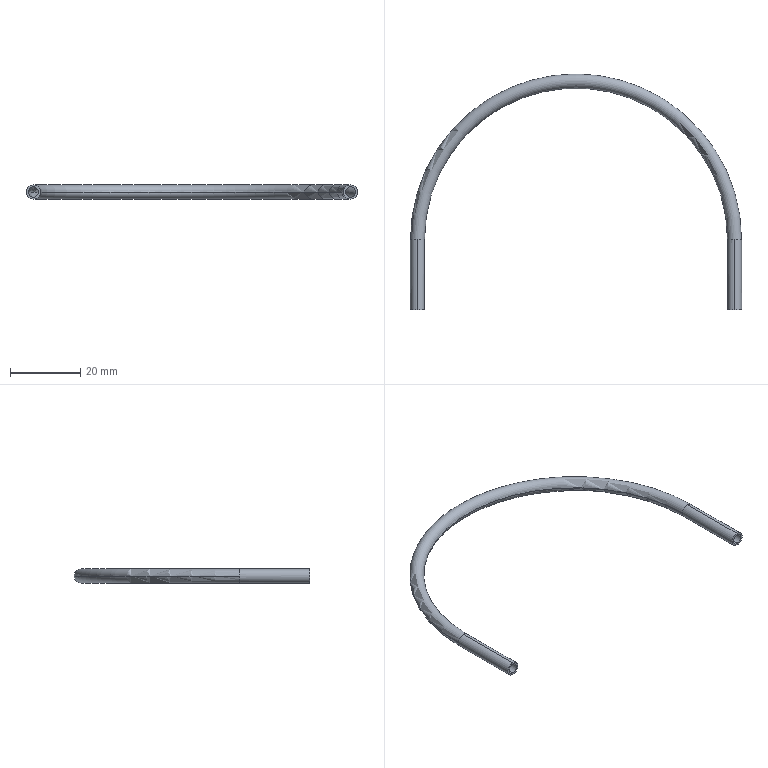Part | STEP file | 1 solid | 14 faces | box 94.3 x 67.15 x 4 mm | volume 999.734 mm3 | cylinder 8 | torus 4 | plane 2 | commonest cylinder face diameters 3 x4 4 x4
STEP:
#1=CARTESIAN_POINT('',(0.,0.,0.));
#2=DIRECTION('',(0.,0.,1.));
#3=DIRECTION('',(1.,0.,0.));
#4=AXIS2_PLACEMENT_3D('',#1,#2,#3);
#5=CARTESIAN_POINT('',(45.15,0.,-2.));
#6=VERTEX_POINT('',#5);
#7=CARTESIAN_POINT('',(45.15,20.,-2.));
#8=VERTEX_POINT('',#7);
#9=CARTESIAN_POINT('',(45.15,0.,-2.));
#10=DIRECTION('',(0.,1.,0.));
#11=VECTOR('',#10,1.);
#12=LINE('',#9,#11);
#13=CARTESIAN_POINT('',(45.15,0.,0.));
#14=DIRECTION('',(0.,1.,0.));
#15=DIRECTION('',(0.,0.,1.));
#16=AXIS2_PLACEMENT_3D('',#13,#14,#15);
#17=CYLINDRICAL_SURFACE('',#16,2.);
#18=CARTESIAN_POINT('',(3.142,0.));
#19=DIRECTION('',(0.,1.));
#20=VECTOR('',#19,1.);
#21=LINE('',#18,#20);
#22=(GEOMETRIC_REPRESENTATION_CONTEXT(2)PARAMETRIC_REPRESENTATION_CONTEXT()REPRESENTATION_CONTEXT('',''));
#23=DEFINITIONAL_REPRESENTATION('',(#21),#22);
#24=PCURVE('',#17,#23);
#25=CARTESIAN_POINT('',(45.15,0.,0.));
#26=DIRECTION('',(0.,1.,0.));
#27=DIRECTION('',(0.,0.,1.));
#28=AXIS2_PLACEMENT_3D('',#25,#26,#27);
#29=CYLINDRICAL_SURFACE('',#28,2.);
#30=CARTESIAN_POINT('',(3.142,0.));
#31=DIRECTION('',(0.,1.));
#32=VECTOR('',#31,1.);
#33=LINE('',#30,#32);
#34=(GEOMETRIC_REPRESENTATION_CONTEXT(2)PARAMETRIC_REPRESENTATION_CONTEXT()REPRESENTATION_CONTEXT('',''));
#35=DEFINITIONAL_REPRESENTATION('',(#33),#34);
#36=PCURVE('',#29,#35);
#37=SURFACE_CURVE('',#12,(#24,#36),.PCURVE_S1.);
#38=EDGE_CURVE('',#6,#8,#37,.T.);
#39=ORIENTED_EDGE('',*,*,#38,.F.);
#40=CARTESIAN_POINT('',(45.15,0.,2.));
#41=VERTEX_POINT('',#40);
#42=CARTESIAN_POINT('',(45.15,0.,0.));
#43=DIRECTION('',(0.,-1.,0.));
#44=DIRECTION('',(0.,0.,1.));
#45=AXIS2_PLACEMENT_3D('',#42,#43,#44);
#46=CIRCLE('',#45,2.);
#47=CARTESIAN_POINT('',(6.283,0.));
#48=DIRECTION('',(-1.,0.));
#49=VECTOR('',#48,1.);
#50=LINE('',#47,#49);
#51=(GEOMETRIC_REPRESENTATION_CONTEXT(2)PARAMETRIC_REPRESENTATION_CONTEXT()REPRESENTATION_CONTEXT('',''));
#52=DEFINITIONAL_REPRESENTATION('',(#50),#51);
#53=PCURVE('',#17,#52);
#54=CARTESIAN_POINT('',(45.15,0.,0.));
#55=DIRECTION('',(0.,-1.,0.));
#56=DIRECTION('',(0.,0.,1.));
#57=AXIS2_PLACEMENT_3D('',#54,#55,#56);
#58=PLANE('',#57);
#59=CARTESIAN_POINT('',(0.,0.));
#60=DIRECTION('',(1.,0.));
#61=AXIS2_PLACEMENT_2D('',#59,#60);
#62=CIRCLE('',#61,2.);
#63=(GEOMETRIC_REPRESENTATION_CONTEXT(2)PARAMETRIC_REPRESENTATION_CONTEXT()REPRESENTATION_CONTEXT('',''));
#64=DEFINITIONAL_REPRESENTATION('',(#62),#63);
#65=PCURVE('',#58,#64);
#66=SURFACE_CURVE('',#46,(#53,#65),.PCURVE_S1.);
#67=EDGE_CURVE('',#41,#6,#66,.T.);
#68=ORIENTED_EDGE('',*,*,#67,.F.);
#69=CARTESIAN_POINT('',(45.15,20.,2.));
#70=VERTEX_POINT('',#69);
#71=CARTESIAN_POINT('',(45.15,0.,2.));
#72=DIRECTION('',(0.,1.,0.));
#73=VECTOR('',#72,1.);
#74=LINE('',#71,#73);
#75=CARTESIAN_POINT('',(6.283,0.));
#76=DIRECTION('',(0.,1.));
#77=VECTOR('',#76,1.);
#78=LINE('',#75,#77);
#79=(GEOMETRIC_REPRESENTATION_CONTEXT(2)PARAMETRIC_REPRESENTATION_CONTEXT()REPRESENTATION_CONTEXT('',''));
#80=DEFINITIONAL_REPRESENTATION('',(#78),#79);
#81=PCURVE('',#17,#80);
#82=CARTESIAN_POINT('',(0.,0.));
#83=DIRECTION('',(0.,1.));
#84=VECTOR('',#83,1.);
#85=LINE('',#82,#84);
#86=(GEOMETRIC_REPRESENTATION_CONTEXT(2)PARAMETRIC_REPRESENTATION_CONTEXT()REPRESENTATION_CONTEXT('',''));
#87=DEFINITIONAL_REPRESENTATION('',(#85),#86);
#88=PCURVE('',#29,#87);
#89=SURFACE_CURVE('',#74,(#81,#88),.PCURVE_S1.);
#90=EDGE_CURVE('',#41,#70,#89,.T.);
#91=ORIENTED_EDGE('',*,*,#90,.T.);
#92=CARTESIAN_POINT('',(43.15,20.,0.));
#93=VERTEX_POINT('',#92);
#94=CARTESIAN_POINT('',(45.15,20.,0.));
#95=DIRECTION('',(0.,-1.,0.));
#96=DIRECTION('',(0.,0.,1.));
#97=AXIS2_PLACEMENT_3D('',#94,#95,#96);
#98=CIRCLE('',#97,2.);
#99=CARTESIAN_POINT('',(6.283,20.));
#100=DIRECTION('',(-1.,0.));
#101=VECTOR('',#100,1.);
#102=LINE('',#99,#101);
#103=(GEOMETRIC_REPRESENTATION_CONTEXT(2)PARAMETRIC_REPRESENTATION_CONTEXT()REPRESENTATION_CONTEXT('',''));
#104=DEFINITIONAL_REPRESENTATION('',(#102),#103);
#105=PCURVE('',#17,#104);
#106=CARTESIAN_POINT('',(0.,20.,0.));
#107=DIRECTION('',(0.,0.,1.));
#108=DIRECTION('',(1.,0.,0.));
#109=AXIS2_PLACEMENT_3D('',#106,#107,#108);
#110=TOROIDAL_SURFACE('',#109,45.15,2.);
#111=CARTESIAN_POINT('',(0.,1.571));
#112=DIRECTION('',(0.,1.));
#113=VECTOR('',#112,1.);
#114=LINE('',#111,#113);
#115=(GEOMETRIC_REPRESENTATION_CONTEXT(2)PARAMETRIC_REPRESENTATION_CONTEXT()REPRESENTATION_CONTEXT('',''));
#116=DEFINITIONAL_REPRESENTATION('',(#114),#115);
#117=PCURVE('',#110,#116);
#118=SURFACE_CURVE('',#98,(#105,#117),.PCURVE_S1.);
#119=EDGE_CURVE('',#70,#93,#118,.T.);
#120=ORIENTED_EDGE('',*,*,#119,.T.);
#121=CARTESIAN_POINT('',(45.15,20.,0.));
#122=DIRECTION('',(0.,-1.,0.));
#123=DIRECTION('',(0.,0.,1.));
#124=AXIS2_PLACEMENT_3D('',#121,#122,#123);
#125=CIRCLE('',#124,2.);
#126=CARTESIAN_POINT('',(6.283,20.));
#127=DIRECTION('',(-1.,0.));
#128=VECTOR('',#127,1.);
#129=LINE('',#126,#128);
#130=(GEOMETRIC_REPRESENTATION_CONTEXT(2)PARAMETRIC_REPRESENTATION_CONTEXT()REPRESENTATION_CONTEXT('',''));
#131=DEFINITIONAL_REPRESENTATION('',(#129),#130);
#132=PCURVE('',#17,#131);
#133=CARTESIAN_POINT('',(0.,20.,0.));
#134=DIRECTION('',(0.,0.,1.));
#135=DIRECTION('',(1.,0.,0.));
#136=AXIS2_PLACEMENT_3D('',#133,#134,#135);
#137=TOROIDAL_SURFACE('',#136,45.15,2.);
#138=CARTESIAN_POINT('',(0.,1.571));
#139=DIRECTION('',(0.,1.));
#140=VECTOR('',#139,1.);
#141=LINE('',#138,#140);
#142=(GEOMETRIC_REPRESENTATION_CONTEXT(2)PARAMETRIC_REPRESENTATION_CONTEXT()REPRESENTATION_CONTEXT('',''));
#143=DEFINITIONAL_REPRESENTATION('',(#141),#142);
#144=PCURVE('',#137,#143);
#145=SURFACE_CURVE('',#125,(#132,#144),.PCURVE_S1.);
#146=EDGE_CURVE('',#93,#8,#145,.T.);
#147=ORIENTED_EDGE('',*,*,#146,.T.);
#148=EDGE_LOOP('',(#39,#68,#91,#120,#147));
#149=FACE_BOUND('',#148,.T.);
#150=ADVANCED_FACE('',(#149),#17,.T.);
#151=CARTESIAN_POINT('',(47.15,20.,0.));
#152=VERTEX_POINT('',#151);
#153=CARTESIAN_POINT('',(-47.15,20.,0.));
#154=VERTEX_POINT('',#153);
#155=CARTESIAN_POINT('',(0.,20.,0.));
#156=DIRECTION('',(0.,0.,1.));
#157=DIRECTION('',(1.,0.,0.));
#158=AXIS2_PLACEMENT_3D('',#155,#156,#157);
#159=CIRCLE('',#158,47.15);
#160=CARTESIAN_POINT('',(0.,6.283));
#161=DIRECTION('',(1.,0.));
#162=VECTOR('',#161,1.);
#163=LINE('',#160,#162);
#164=(GEOMETRIC_REPRESENTATION_CONTEXT(2)PARAMETRIC_REPRESENTATION_CONTEXT()REPRESENTATION_CONTEXT('',''));
#165=DEFINITIONAL_REPRESENTATION('',(#163),#164);
#166=PCURVE('',#137,#165);
#167=CARTESIAN_POINT('',(0.,0.));
#168=DIRECTION('',(1.,0.));
#169=VECTOR('',#168,1.);
#170=LINE('',#167,#169);
#171=(GEOMETRIC_REPRESENTATION_CONTEXT(2)PARAMETRIC_REPRESENTATION_CONTEXT()REPRESENTATION_CONTEXT('',''));
#172=DEFINITIONAL_REPRESENTATION('',(#170),#171);
#173=PCURVE('',#110,#172);
#174=SURFACE_CURVE('',#159,(#166,#173),.PCURVE_S1.);
#175=EDGE_CURVE('',#152,#154,#174,.T.);
#176=ORIENTED_EDGE('',*,*,#175,.F.);
#177=CARTESIAN_POINT('',(45.15,20.,0.));
#178=DIRECTION('',(0.,-1.,0.));
#179=DIRECTION('',(0.,0.,1.));
#180=AXIS2_PLACEMENT_3D('',#177,#178,#179);
#181=CIRCLE('',#180,2.);
#182=CARTESIAN_POINT('',(0.,1.571));
#183=DIRECTION('',(0.,1.));
#184=VECTOR('',#183,1.);
#185=LINE('',#182,#184);
#186=(GEOMETRIC_REPRESENTATION_CONTEXT(2)PARAMETRIC_REPRESENTATION_CONTEXT()REPRESENTATION_CONTEXT('',''));
#187=DEFINITIONAL_REPRESENTATION('',(#185),#186);
#188=PCURVE('',#137,#187);
#189=CARTESIAN_POINT('',(6.283,20.));
#190=DIRECTION('',(-1.,0.));
#191=VECTOR('',#190,1.);
#192=LINE('',#189,#191);
#193=(GEOMETRIC_REPRESENTATION_CONTEXT(2)PARAMETRIC_REPRESENTATION_CONTEXT()REPRESENTATION_CONTEXT('',''));
#194=DEFINITIONAL_REPRESENTATION('',(#192),#193);
#195=PCURVE('',#29,#194);
#196=SURFACE_CURVE('',#181,(#188,#195),.PCURVE_S1.);
#197=EDGE_CURVE('',#8,#152,#196,.T.);
#198=ORIENTED_EDGE('',*,*,#197,.F.);
#199=ORIENTED_EDGE('',*,*,#146,.F.);
#200=CARTESIAN_POINT('',(-43.15,20.,0.));
#201=VERTEX_POINT('',#200);
#202=CARTESIAN_POINT('',(0.,20.,0.));
#203=DIRECTION('',(0.,0.,1.));
#204=DIRECTION('',(1.,0.,0.));
#205=AXIS2_PLACEMENT_3D('',#202,#203,#204);
#206=CIRCLE('',#205,43.15);
#207=CARTESIAN_POINT('',(0.,3.142));
#208=DIRECTION('',(1.,0.));
#209=VECTOR('',#208,1.);
#210=LINE('',#207,#209);
#211=(GEOMETRIC_REPRESENTATION_CONTEXT(2)PARAMETRIC_REPRESENTATION_CONTEXT()REPRESENTATION_CONTEXT('',''));
#212=DEFINITIONAL_REPRESENTATION('',(#210),#211);
#213=PCURVE('',#137,#212);
#214=CARTESIAN_POINT('',(0.,3.142));
#215=DIRECTION('',(1.,0.));
#216=VECTOR('',#215,1.);
#217=LINE('',#214,#216);
#218=(GEOMETRIC_REPRESENTATION_CONTEXT(2)PARAMETRIC_REPRESENTATION_CONTEXT()REPRESENTATION_CONTEXT('',''));
#219=DEFINITIONAL_REPRESENTATION('',(#217),#218);
#220=PCURVE('',#110,#219);
#221=SURFACE_CURVE('',#206,(#213,#220),.PCURVE_S1.);
#222=EDGE_CURVE('',#93,#201,#221,.T.);
#223=ORIENTED_EDGE('',*,*,#222,.T.);
#224=CARTESIAN_POINT('',(-45.15,20.,-2.));
#225=VERTEX_POINT('',#224);
#226=CARTESIAN_POINT('',(-45.15,20.,0.));
#227=DIRECTION('',(0.,1.,0.));
#228=DIRECTION('',(0.,0.,1.));
#229=AXIS2_PLACEMENT_3D('',#226,#227,#228);
#230=CIRCLE('',#229,2.);
#231=CARTESIAN_POINT('',(3.142,1.571));
#232=DIRECTION('',(0.,1.));
#233=VECTOR('',#232,1.);
#234=LINE('',#231,#233);
#235=(GEOMETRIC_REPRESENTATION_CONTEXT(2)PARAMETRIC_REPRESENTATION_CONTEXT()REPRESENTATION_CONTEXT('',''));
#236=DEFINITIONAL_REPRESENTATION('',(#234),#235);
#237=PCURVE('',#137,#236);
#238=CARTESIAN_POINT('',(-45.15,20.,0.));
#239=DIRECTION('',(0.,-1.,0.));
#240=DIRECTION('',(0.,0.,-1.));
#241=AXIS2_PLACEMENT_3D('',#238,#239,#240);
#242=CYLINDRICAL_SURFACE('',#241,2.);
#243=CARTESIAN_POINT('',(3.142,0.));
#244=DIRECTION('',(-1.,0.));
#245=VECTOR('',#244,1.);
#246=LINE('',#243,#245);
#247=(GEOMETRIC_REPRESENTATION_CONTEXT(2)PARAMETRIC_REPRESENTATION_CONTEXT()REPRESENTATION_CONTEXT('',''));
#248=DEFINITIONAL_REPRESENTATION('',(#246),#247);
#249=PCURVE('',#242,#248);
#250=SURFACE_CURVE('',#230,(#237,#249),.PCURVE_S1.);
#251=EDGE_CURVE('',#201,#225,#250,.T.);
#252=ORIENTED_EDGE('',*,*,#251,.T.);
#253=CARTESIAN_POINT('',(-45.15,20.,0.));
#254=DIRECTION('',(0.,1.,0.));
#255=DIRECTION('',(0.,0.,1.));
#256=AXIS2_PLACEMENT_3D('',#253,#254,#255);
#257=CIRCLE('',#256,2.);
#258=CARTESIAN_POINT('',(3.142,1.571));
#259=DIRECTION('',(0.,1.));
#260=VECTOR('',#259,1.);
#261=LINE('',#258,#260);
#262=(GEOMETRIC_REPRESENTATION_CONTEXT(2)PARAMETRIC_REPRESENTATION_CONTEXT()REPRESENTATION_CONTEXT('',''));
#263=DEFINITIONAL_REPRESENTATION('',(#261),#262);
#264=PCURVE('',#137,#263);
#265=CARTESIAN_POINT('',(-45.15,20.,0.));
#266=DIRECTION('',(0.,-1.,0.));
#267=DIRECTION('',(0.,0.,-1.));
#268=AXIS2_PLACEMENT_3D('',#265,#266,#267);
#269=CYLINDRICAL_SURFACE('',#268,2.);
#270=CARTESIAN_POINT('',(9.425,0.));
#271=DIRECTION('',(-1.,0.));
#272=VECTOR('',#271,1.);
#273=LINE('',#270,#272);
#274=(GEOMETRIC_REPRESENTATION_CONTEXT(2)PARAMETRIC_REPRESENTATION_CONTEXT()REPRESENTATION_CONTEXT('',''));
#275=DEFINITIONAL_REPRESENTATION('',(#273),#274);
#276=PCURVE('',#269,#275);
#277=SURFACE_CURVE('',#257,(#264,#276),.PCURVE_S1.);
#278=EDGE_CURVE('',#225,#154,#277,.T.);
#279=ORIENTED_EDGE('',*,*,#278,.T.);
#280=EDGE_LOOP('',(#176,#198,#199,#223,#252,#279));
#281=FACE_BOUND('',#280,.T.);
#282=ADVANCED_FACE('',(#281),#137,.T.);
#283=CARTESIAN_POINT('',(-45.15,20.,2.));
#284=VERTEX_POINT('',#283);
#285=CARTESIAN_POINT('',(-45.15,0.,2.));
#286=VERTEX_POINT('',#285);
#287=CARTESIAN_POINT('',(-45.15,20.,2.));
#288=DIRECTION('',(0.,-1.,0.));
#289=VECTOR('',#288,1.);
#290=LINE('',#287,#289);
#291=CARTESIAN_POINT('',(3.142,0.));
#292=DIRECTION('',(0.,1.));
#293=VECTOR('',#292,1.);
#294=LINE('',#291,#293);
#295=(GEOMETRIC_REPRESENTATION_CONTEXT(2)PARAMETRIC_REPRESENTATION_CONTEXT()REPRESENTATION_CONTEXT('',''));
#296=DEFINITIONAL_REPRESENTATION('',(#294),#295);
#297=PCURVE('',#269,#296);
#298=CARTESIAN_POINT('',(3.142,0.));
#299=DIRECTION('',(0.,1.));
#300=VECTOR('',#299,1.);
#301=LINE('',#298,#300);
#302=(GEOMETRIC_REPRESENTATION_CONTEXT(2)PARAMETRIC_REPRESENTATION_CONTEXT()REPRESENTATION_CONTEXT('',''));
#303=DEFINITIONAL_REPRESENTATION('',(#301),#302);
#304=PCURVE('',#242,#303);
#305=SURFACE_CURVE('',#290,(#297,#304),.PCURVE_S1.);
#306=EDGE_CURVE('',#284,#286,#305,.T.);
#307=ORIENTED_EDGE('',*,*,#306,.F.);
#308=CARTESIAN_POINT('',(-45.15,20.,0.));
#309=DIRECTION('',(0.,1.,0.));
#310=DIRECTION('',(0.,0.,1.));
#311=AXIS2_PLACEMENT_3D('',#308,#309,#310);
#312=CIRCLE('',#311,2.);
#313=CARTESIAN_POINT('',(9.425,0.));
#314=DIRECTION('',(-1.,0.));
#315=VECTOR('',#314,1.);
#316=LINE('',#313,#315);
#317=(GEOMETRIC_REPRESENTATION_CONTEXT(2)PARAMETRIC_REPRESENTATION_CONTEXT()REPRESENTATION_CONTEXT('',''));
#318=DEFINITIONAL_REPRESENTATION('',(#316),#317);
#319=PCURVE('',#269,#318);
#320=CARTESIAN_POINT('',(3.142,-4.712));
#321=DIRECTION('',(0.,1.));
#322=VECTOR('',#321,1.);
#323=LINE('',#320,#322);
#324=(GEOMETRIC_REPRESENTATION_CONTEXT(2)PARAMETRIC_REPRESENTATION_CONTEXT()REPRESENTATION_CONTEXT('',''));
#325=DEFINITIONAL_REPRESENTATION('',(#323),#324);
#326=PCURVE('',#110,#325);
#327=SURFACE_CURVE('',#312,(#319,#326),.PCURVE_S1.);
#328=EDGE_CURVE('',#154,#284,#327,.T.);
#329=ORIENTED_EDGE('',*,*,#328,.F.);
#330=ORIENTED_EDGE('',*,*,#278,.F.);
#331=CARTESIAN_POINT('',(-45.15,0.,-2.));
#332=VERTEX_POINT('',#331);
#333=CARTESIAN_POINT('',(-45.15,20.,-2.));
#334=DIRECTION('',(0.,-1.,0.));
#335=VECTOR('',#334,1.);
#336=LINE('',#333,#335);
#337=CARTESIAN_POINT('',(6.283,0.));
#338=DIRECTION('',(0.,1.));
#339=VECTOR('',#338,1.);
#340=LINE('',#337,#339);
#341=(GEOMETRIC_REPRESENTATION_CONTEXT(2)PARAMETRIC_REPRESENTATION_CONTEXT()REPRESENTATION_CONTEXT('',''));
#342=DEFINITIONAL_REPRESENTATION('',(#340),#341);
#343=PCURVE('',#269,#342);
#344=CARTESIAN_POINT('',(0.,0.));
#345=DIRECTION('',(0.,1.));
#346=VECTOR('',#345,1.);
#347=LINE('',#344,#346);
#348=(GEOMETRIC_REPRESENTATION_CONTEXT(2)PARAMETRIC_REPRESENTATION_CONTEXT()REPRESENTATION_CONTEXT('',''));
#349=DEFINITIONAL_REPRESENTATION('',(#347),#348);
#350=PCURVE('',#242,#349);
#351=SURFACE_CURVE('',#336,(#343,#350),.PCURVE_S1.);
#352=EDGE_CURVE('',#225,#332,#351,.T.);
#353=ORIENTED_EDGE('',*,*,#352,.T.);
#354=CARTESIAN_POINT('',(-45.15,0.,0.));
#355=DIRECTION('',(0.,1.,0.));
#356=DIRECTION('',(0.,0.,1.));
#357=AXIS2_PLACEMENT_3D('',#354,#355,#356);
#358=CIRCLE('',#357,2.);
#359=CARTESIAN_POINT('',(9.425,20.));
#360=DIRECTION('',(-1.,0.));
#361=VECTOR('',#360,1.);
#362=LINE('',#359,#361);
#363=(GEOMETRIC_REPRESENTATION_CONTEXT(2)PARAMETRIC_REPRESENTATION_CONTEXT()REPRESENTATION_CONTEXT('',''));
#364=DEFINITIONAL_REPRESENTATION('',(#362),#363);
#365=PCURVE('',#269,#364);
#366=CARTESIAN_POINT('',(-45.15,0.,0.));
#367=DIRECTION('',(0.,1.,0.));
#368=DIRECTION('',(0.,0.,1.));
#369=AXIS2_PLACEMENT_3D('',#366,#367,#368);
#370=PLANE('',#369);
#371=CARTESIAN_POINT('',(0.,0.));
#372=DIRECTION('',(1.,0.));
#373=AXIS2_PLACEMENT_2D('',#371,#372);
#374=CIRCLE('',#373,2.);
#375=(GEOMETRIC_REPRESENTATION_CONTEXT(2)PARAMETRIC_REPRESENTATION_CONTEXT()REPRESENTATION_CONTEXT('',''));
#376=DEFINITIONAL_REPRESENTATION('',(#374),#375);
#377=PCURVE('',#370,#376);
#378=SURFACE_CURVE('',#358,(#365,#377),.PCURVE_S1.);
#379=EDGE_CURVE('',#332,#286,#378,.T.);
#380=ORIENTED_EDGE('',*,*,#379,.T.);
#381=EDGE_LOOP('',(#307,#329,#330,#353,#380));
#382=FACE_BOUND('',#381,.T.);
#383=ADVANCED_FACE('',(#382),#269,.T.);
#384=ORIENTED_EDGE('',*,*,#67,.T.);
#385=CARTESIAN_POINT('',(45.15,0.,0.));
#386=DIRECTION('',(0.,-1.,0.));
#387=DIRECTION('',(0.,0.,1.));
#388=AXIS2_PLACEMENT_3D('',#385,#386,#387);
#389=CIRCLE('',#388,2.);
#390=CARTESIAN_POINT('',(0.,0.));
#391=DIRECTION('',(1.,0.));
#392=AXIS2_PLACEMENT_2D('',#390,#391);
#393=CIRCLE('',#392,2.);
#394=(GEOMETRIC_REPRESENTATION_CONTEXT(2)PARAMETRIC_REPRESENTATION_CONTEXT()REPRESENTATION_CONTEXT('',''));
#395=DEFINITIONAL_REPRESENTATION('',(#393),#394);
#396=PCURVE('',#58,#395);
#397=CARTESIAN_POINT('',(6.283,0.));
#398=DIRECTION('',(-1.,0.));
#399=VECTOR('',#398,1.);
#400=LINE('',#397,#399);
#401=(GEOMETRIC_REPRESENTATION_CONTEXT(2)PARAMETRIC_REPRESENTATION_CONTEXT()REPRESENTATION_CONTEXT('',''));
#402=DEFINITIONAL_REPRESENTATION('',(#400),#401);
#403=PCURVE('',#29,#402);
#404=SURFACE_CURVE('',#389,(#396,#403),.PCURVE_S1.);
#405=EDGE_CURVE('',#6,#41,#404,.T.);
#406=ORIENTED_EDGE('',*,*,#405,.T.);
#407=EDGE_LOOP('',(#384,#406));
#408=FACE_BOUND('',#407,.T.);
#409=CARTESIAN_POINT('',(45.15,0.,1.5));
#410=VERTEX_POINT('',#409);
#411=CARTESIAN_POINT('',(45.15,0.,-1.5));
#412=VERTEX_POINT('',#411);
#413=CARTESIAN_POINT('',(45.15,0.,0.));
#414=DIRECTION('',(0.,1.,0.));
#415=DIRECTION('',(0.,0.,1.));
#416=AXIS2_PLACEMENT_3D('',#413,#414,#415);
#417=CIRCLE('',#416,1.5);
#418=CARTESIAN_POINT('',(1.5,0.));
#419=CARTESIAN_POINT('',(1.5,-2.598));
#420=CARTESIAN_POINT('',(-0.75,-1.299));
#421=CARTESIAN_POINT('',(-3.,0.));
#422=CARTESIAN_POINT('',(-0.75,1.299));
#423=CARTESIAN_POINT('',(1.5,2.598));
#424=CARTESIAN_POINT('',(1.5,0.));
#425=(BOUNDED_CURVE()B_SPLINE_CURVE(2,(#418,#419,#420,#421,#422,#423,#424),.UNSPECIFIED.,.T.,.F.)B_SPLINE_CURVE_WITH_KNOTS((1,2,2,2,2,1),(-2.094,0.,2.094,4.189,6.283,8.378),.UNSPECIFIED.)CURVE()GEOMETRIC_REPRESENTATION_ITEM()RATIONAL_B_SPLINE_CURVE((1.,0.5,1.,0.5,1.,0.5,1.))REPRESENTATION_ITEM(''));
#426=(GEOMETRIC_REPRESENTATION_CONTEXT(2)PARAMETRIC_REPRESENTATION_CONTEXT()REPRESENTATION_CONTEXT('',''));
#427=DEFINITIONAL_REPRESENTATION('',(#425),#426);
#428=PCURVE('',#58,#427);
#429=CARTESIAN_POINT('',(45.15,0.,0.));
#430=DIRECTION('',(0.,1.,0.));
#431=DIRECTION('',(0.,0.,1.));
#432=AXIS2_PLACEMENT_3D('',#429,#430,#431);
#433=CYLINDRICAL_SURFACE('',#432,1.5);
#434=CARTESIAN_POINT('',(0.,0.));
#435=DIRECTION('',(1.,0.));
#436=VECTOR('',#435,1.);
#437=LINE('',#434,#436);
#438=(GEOMETRIC_REPRESENTATION_CONTEXT(2)PARAMETRIC_REPRESENTATION_CONTEXT()REPRESENTATION_CONTEXT('',''));
#439=DEFINITIONAL_REPRESENTATION('',(#437),#438);
#440=PCURVE('',#433,#439);
#441=SURFACE_CURVE('',#417,(#428,#440),.PCURVE_S1.);
#442=EDGE_CURVE('',#410,#412,#441,.T.);
#443=ORIENTED_EDGE('',*,*,#442,.T.);
#444=CARTESIAN_POINT('',(45.15,0.,0.));
#445=DIRECTION('',(0.,1.,0.));
#446=DIRECTION('',(0.,0.,1.));
#447=AXIS2_PLACEMENT_3D('',#444,#445,#446);
#448=CIRCLE('',#447,1.5);
#449=CARTESIAN_POINT('',(1.5,0.));
#450=CARTESIAN_POINT('',(1.5,-2.598));
#451=CARTESIAN_POINT('',(-0.75,-1.299));
#452=CARTESIAN_POINT('',(-3.,0.));
#453=CARTESIAN_POINT('',(-0.75,1.299));
#454=CARTESIAN_POINT('',(1.5,2.598));
#455=CARTESIAN_POINT('',(1.5,0.));
#456=(BOUNDED_CURVE()B_SPLINE_CURVE(2,(#449,#450,#451,#452,#453,#454,#455),.UNSPECIFIED.,.T.,.F.)B_SPLINE_CURVE_WITH_KNOTS((1,2,2,2,2,1),(-2.094,0.,2.094,4.189,6.283,8.378),.UNSPECIFIED.)CURVE()GEOMETRIC_REPRESENTATION_ITEM()RATIONAL_B_SPLINE_CURVE((1.,0.5,1.,0.5,1.,0.5,1.))REPRESENTATION_ITEM(''));
#457=(GEOMETRIC_REPRESENTATION_CONTEXT(2)PARAMETRIC_REPRESENTATION_CONTEXT()REPRESENTATION_CONTEXT('',''));
#458=DEFINITIONAL_REPRESENTATION('',(#456),#457);
#459=PCURVE('',#58,#458);
#460=CARTESIAN_POINT('',(45.15,0.,0.));
#461=DIRECTION('',(0.,1.,0.));
#462=DIRECTION('',(0.,0.,1.));
#463=AXIS2_PLACEMENT_3D('',#460,#461,#462);
#464=CYLINDRICAL_SURFACE('',#463,1.5);
#465=CARTESIAN_POINT('',(0.,0.));
#466=DIRECTION('',(1.,0.));
#467=VECTOR('',#466,1.);
#468=LINE('',#465,#467);
#469=(GEOMETRIC_REPRESENTATION_CONTEXT(2)PARAMETRIC_REPRESENTATION_CONTEXT()REPRESENTATION_CONTEXT('',''));
#470=DEFINITIONAL_REPRESENTATION('',(#468),#469);
#471=PCURVE('',#464,#470);
#472=SURFACE_CURVE('',#448,(#459,#471),.PCURVE_S1.);
#473=EDGE_CURVE('',#412,#410,#472,.T.);
#474=ORIENTED_EDGE('',*,*,#473,.T.);
#475=EDGE_LOOP('',(#443,#474));
#476=FACE_BOUND('',#475,.T.);
#477=ADVANCED_FACE('',(#408,#476),#58,.T.);
#478=ORIENTED_EDGE('',*,*,#379,.F.);
#479=CARTESIAN_POINT('',(-45.15,0.,0.));
#480=DIRECTION('',(0.,1.,0.));
#481=DIRECTION('',(0.,0.,1.));
#482=AXIS2_PLACEMENT_3D('',#479,#480,#481);
#483=CIRCLE('',#482,2.);
#484=CARTESIAN_POINT('',(0.,0.));
#485=DIRECTION('',(1.,0.));
#486=AXIS2_PLACEMENT_2D('',#484,#485);
#487=CIRCLE('',#486,2.);
#488=(GEOMETRIC_REPRESENTATION_CONTEXT(2)PARAMETRIC_REPRESENTATION_CONTEXT()REPRESENTATION_CONTEXT('',''));
#489=DEFINITIONAL_REPRESENTATION('',(#487),#488);
#490=PCURVE('',#370,#489);
#491=CARTESIAN_POINT('',(3.142,20.));
#492=DIRECTION('',(-1.,0.));
#493=VECTOR('',#492,1.);
#494=LINE('',#491,#493);
#495=(GEOMETRIC_REPRESENTATION_CONTEXT(2)PARAMETRIC_REPRESENTATION_CONTEXT()REPRESENTATION_CONTEXT('',''));
#496=DEFINITIONAL_REPRESENTATION('',(#494),#495);
#497=PCURVE('',#242,#496);
#498=SURFACE_CURVE('',#483,(#490,#497),.PCURVE_S1.);
#499=EDGE_CURVE('',#286,#332,#498,.T.);
#500=ORIENTED_EDGE('',*,*,#499,.F.);
#501=EDGE_LOOP('',(#478,#500));
#502=FACE_BOUND('',#501,.T.);
#503=CARTESIAN_POINT('',(-45.15,0.,-1.5));
#504=VERTEX_POINT('',#503);
#505=CARTESIAN_POINT('',(-45.15,0.,1.5));
#506=VERTEX_POINT('',#505);
#507=CARTESIAN_POINT('',(-45.15,0.,0.));
#508=DIRECTION('',(0.,-1.,0.));
#509=DIRECTION('',(0.,0.,1.));
#510=AXIS2_PLACEMENT_3D('',#507,#508,#509);
#511=CIRCLE('',#510,1.5);
#512=CARTESIAN_POINT('',(1.5,0.));
#513=CARTESIAN_POINT('',(1.5,-2.598));
#514=CARTESIAN_POINT('',(-0.75,-1.299));
#515=CARTESIAN_POINT('',(-3.,0.));
#516=CARTESIAN_POINT('',(-0.75,1.299));
#517=CARTESIAN_POINT('',(1.5,2.598));
#518=CARTESIAN_POINT('',(1.5,0.));
#519=(BOUNDED_CURVE()B_SPLINE_CURVE(2,(#512,#513,#514,#515,#516,#517,#518),.UNSPECIFIED.,.T.,.F.)B_SPLINE_CURVE_WITH_KNOTS((1,2,2,2,2,1),(-2.094,0.,2.094,4.189,6.283,8.378),.UNSPECIFIED.)CURVE()GEOMETRIC_REPRESENTATION_ITEM()RATIONAL_B_SPLINE_CURVE((1.,0.5,1.,0.5,1.,0.5,1.))REPRESENTATION_ITEM(''));
#520=(GEOMETRIC_REPRESENTATION_CONTEXT(2)PARAMETRIC_REPRESENTATION_CONTEXT()REPRESENTATION_CONTEXT('',''));
#521=DEFINITIONAL_REPRESENTATION('',(#519),#520);
#522=PCURVE('',#370,#521);
#523=CARTESIAN_POINT('',(-45.15,20.,0.));
#524=DIRECTION('',(0.,-1.,0.));
#525=DIRECTION('',(0.,0.,-1.));
#526=AXIS2_PLACEMENT_3D('',#523,#524,#525);
#527=CYLINDRICAL_SURFACE('',#526,1.5);
#528=CARTESIAN_POINT('',(-3.142,20.));
#529=DIRECTION('',(1.,0.));
#530=VECTOR('',#529,1.);
#531=LINE('',#528,#530);
#532=(GEOMETRIC_REPRESENTATION_CONTEXT(2)PARAMETRIC_REPRESENTATION_CONTEXT()REPRESENTATION_CONTEXT('',''));
#533=DEFINITIONAL_REPRESENTATION('',(#531),#532);
#534=PCURVE('',#527,#533);
#535=SURFACE_CURVE('',#511,(#522,#534),.PCURVE_S1.);
#536=EDGE_CURVE('',#504,#506,#535,.T.);
#537=ORIENTED_EDGE('',*,*,#536,.F.);
#538=CARTESIAN_POINT('',(-45.15,0.,0.));
#539=DIRECTION('',(0.,-1.,0.));
#540=DIRECTION('',(0.,0.,1.));
#541=AXIS2_PLACEMENT_3D('',#538,#539,#540);
#542=CIRCLE('',#541,1.5);
#543=CARTESIAN_POINT('',(1.5,0.));
#544=CARTESIAN_POINT('',(1.5,-2.598));
#545=CARTESIAN_POINT('',(-0.75,-1.299));
#546=CARTESIAN_POINT('',(-3.,0.));
#547=CARTESIAN_POINT('',(-0.75,1.299));
#548=CARTESIAN_POINT('',(1.5,2.598));
#549=CARTESIAN_POINT('',(1.5,0.));
#550=(BOUNDED_CURVE()B_SPLINE_CURVE(2,(#543,#544,#545,#546,#547,#548,#549),.UNSPECIFIED.,.T.,.F.)B_SPLINE_CURVE_WITH_KNOTS((1,2,2,2,2,1),(-2.094,0.,2.094,4.189,6.283,8.378),.UNSPECIFIED.)CURVE()GEOMETRIC_REPRESENTATION_ITEM()RATIONAL_B_SPLINE_CURVE((1.,0.5,1.,0.5,1.,0.5,1.))REPRESENTATION_ITEM(''));
#551=(GEOMETRIC_REPRESENTATION_CONTEXT(2)PARAMETRIC_REPRESENTATION_CONTEXT()REPRESENTATION_CONTEXT('',''));
#552=DEFINITIONAL_REPRESENTATION('',(#550),#551);
#553=PCURVE('',#370,#552);
#554=CARTESIAN_POINT('',(-45.15,20.,0.));
#555=DIRECTION('',(0.,-1.,0.));
#556=DIRECTION('',(0.,0.,-1.));
#557=AXIS2_PLACEMENT_3D('',#554,#555,#556);
#558=CYLINDRICAL_SURFACE('',#557,1.5);
#559=CARTESIAN_POINT('',(3.142,20.));
#560=DIRECTION('',(1.,0.));
#561=VECTOR('',#560,1.);
#562=LINE('',#559,#561);
#563=(GEOMETRIC_REPRESENTATION_CONTEXT(2)PARAMETRIC_REPRESENTATION_CONTEXT()REPRESENTATION_CONTEXT('',''));
#564=DEFINITIONAL_REPRESENTATION('',(#562),#563);
#565=PCURVE('',#558,#564);
#566=SURFACE_CURVE('',#542,(#553,#565),.PCURVE_S1.);
#567=EDGE_CURVE('',#506,#504,#566,.T.);
#568=ORIENTED_EDGE('',*,*,#567,.F.);
#569=EDGE_LOOP('',(#537,#568));
#570=FACE_BOUND('',#569,.T.);
#571=ADVANCED_FACE('',(#502,#570),#370,.F.);
#572=CARTESIAN_POINT('',(46.65,20.,0.));
#573=VERTEX_POINT('',#572);
#574=CARTESIAN_POINT('',(45.15,20.,-1.5));
#575=VERTEX_POINT('',#574);
#576=CARTESIAN_POINT('',(45.15,20.,0.));
#577=DIRECTION('',(0.,1.,0.));
#578=DIRECTION('',(0.,0.,1.));
#579=AXIS2_PLACEMENT_3D('',#576,#577,#578);
#580=CIRCLE('',#579,1.5);
#581=CARTESIAN_POINT('',(0.,20.));
#582=DIRECTION('',(1.,0.));
#583=VECTOR('',#582,1.);
#584=LINE('',#581,#583);
#585=(GEOMETRIC_REPRESENTATION_CONTEXT(2)PARAMETRIC_REPRESENTATION_CONTEXT()REPRESENTATION_CONTEXT('',''));
#586=DEFINITIONAL_REPRESENTATION('',(#584),#585);
#587=PCURVE('',#433,#586);
#588=CARTESIAN_POINT('',(0.,20.,0.));
#589=DIRECTION('',(0.,0.,1.));
#590=DIRECTION('',(1.,0.,0.));
#591=AXIS2_PLACEMENT_3D('',#588,#589,#590);
#592=TOROIDAL_SURFACE('',#591,45.15,1.5);
#593=CARTESIAN_POINT('',(0.,7.854));
#594=DIRECTION('',(0.,-1.));
#595=VECTOR('',#594,1.);
#596=LINE('',#593,#595);
#597=(GEOMETRIC_REPRESENTATION_CONTEXT(2)PARAMETRIC_REPRESENTATION_CONTEXT()REPRESENTATION_CONTEXT('',''));
#598=DEFINITIONAL_REPRESENTATION('',(#596),#597);
#599=PCURVE('',#592,#598);
#600=SURFACE_CURVE('',#580,(#587,#599),.PCURVE_S1.);
#601=EDGE_CURVE('',#573,#575,#600,.T.);
#602=ORIENTED_EDGE('',*,*,#601,.F.);
#603=CARTESIAN_POINT('',(45.15,20.,1.5));
#604=VERTEX_POINT('',#603);
#605=CARTESIAN_POINT('',(45.15,20.,0.));
#606=DIRECTION('',(0.,1.,0.));
#607=DIRECTION('',(0.,0.,1.));
#608=AXIS2_PLACEMENT_3D('',#605,#606,#607);
#609=CIRCLE('',#608,1.5);
#610=CARTESIAN_POINT('',(0.,20.));
#611=DIRECTION('',(1.,0.));
#612=VECTOR('',#611,1.);
#613=LINE('',#610,#612);
#614=(GEOMETRIC_REPRESENTATION_CONTEXT(2)PARAMETRIC_REPRESENTATION_CONTEXT()REPRESENTATION_CONTEXT('',''));
#615=DEFINITIONAL_REPRESENTATION('',(#613),#614);
#616=PCURVE('',#433,#615);
#617=CARTESIAN_POINT('',(0.,20.,0.));
#618=DIRECTION('',(0.,0.,1.));
#619=DIRECTION('',(1.,0.,0.));
#620=AXIS2_PLACEMENT_3D('',#617,#618,#619);
#621=TOROIDAL_SURFACE('',#620,45.15,1.5);
#622=CARTESIAN_POINT('',(0.,1.571));
#623=DIRECTION('',(0.,-1.));
#624=VECTOR('',#623,1.);
#625=LINE('',#622,#624);
#626=(GEOMETRIC_REPRESENTATION_CONTEXT(2)PARAMETRIC_REPRESENTATION_CONTEXT()REPRESENTATION_CONTEXT('',''));
#627=DEFINITIONAL_REPRESENTATION('',(#625),#626);
#628=PCURVE('',#621,#627);
#629=SURFACE_CURVE('',#609,(#616,#628),.PCURVE_S1.);
#630=EDGE_CURVE('',#604,#573,#629,.T.);
#631=ORIENTED_EDGE('',*,*,#630,.F.);
#632=CARTESIAN_POINT('',(45.15,0.,1.5));
#633=DIRECTION('',(0.,1.,0.));
#634=VECTOR('',#633,1.);
#635=LINE('',#632,#634);
#636=CARTESIAN_POINT('',(0.,0.));
#637=DIRECTION('',(0.,1.));
#638=VECTOR('',#637,1.);
#639=LINE('',#636,#638);
#640=(GEOMETRIC_REPRESENTATION_CONTEXT(2)PARAMETRIC_REPRESENTATION_CONTEXT()REPRESENTATION_CONTEXT('',''));
#641=DEFINITIONAL_REPRESENTATION('',(#639),#640);
#642=PCURVE('',#433,#641);
#643=CARTESIAN_POINT('',(6.283,0.));
#644=DIRECTION('',(0.,1.));
#645=VECTOR('',#644,1.);
#646=LINE('',#643,#645);
#647=(GEOMETRIC_REPRESENTATION_CONTEXT(2)PARAMETRIC_REPRESENTATION_CONTEXT()REPRESENTATION_CONTEXT('',''));
#648=DEFINITIONAL_REPRESENTATION('',(#646),#647);
#649=PCURVE('',#464,#648);
#650=SURFACE_CURVE('',#635,(#642,#649),.PCURVE_S1.);
#651=EDGE_CURVE('',#410,#604,#650,.T.);
#652=ORIENTED_EDGE('',*,*,#651,.F.);
#653=ORIENTED_EDGE('',*,*,#442,.T.);
#654=CARTESIAN_POINT('',(45.15,0.,-1.5));
#655=DIRECTION('',(0.,1.,0.));
#656=VECTOR('',#655,1.);
#657=LINE('',#654,#656);
#658=CARTESIAN_POINT('',(3.142,0.));
#659=DIRECTION('',(0.,1.));
#660=VECTOR('',#659,1.);
#661=LINE('',#658,#660);
#662=(GEOMETRIC_REPRESENTATION_CONTEXT(2)PARAMETRIC_REPRESENTATION_CONTEXT()REPRESENTATION_CONTEXT('',''));
#663=DEFINITIONAL_REPRESENTATION('',(#661),#662);
#664=PCURVE('',#433,#663);
#665=CARTESIAN_POINT('',(3.142,0.));
#666=DIRECTION('',(0.,1.));
#667=VECTOR('',#666,1.);
#668=LINE('',#665,#667);
#669=(GEOMETRIC_REPRESENTATION_CONTEXT(2)PARAMETRIC_REPRESENTATION_CONTEXT()REPRESENTATION_CONTEXT('',''));
#670=DEFINITIONAL_REPRESENTATION('',(#668),#669);
#671=PCURVE('',#464,#670);
#672=SURFACE_CURVE('',#657,(#664,#671),.PCURVE_S1.);
#673=EDGE_CURVE('',#412,#575,#672,.T.);
#674=ORIENTED_EDGE('',*,*,#673,.T.);
#675=EDGE_LOOP('',(#602,#631,#652,#653,#674));
#676=FACE_BOUND('',#675,.F.);
#677=ADVANCED_FACE('',(#676),#433,.F.);
#678=CARTESIAN_POINT('',(-45.15,20.,1.5));
#679=VERTEX_POINT('',#678);
#680=CARTESIAN_POINT('',(-46.65,20.,0.));
#681=VERTEX_POINT('',#680);
#682=CARTESIAN_POINT('',(-45.15,20.,0.));
#683=DIRECTION('',(0.,-1.,0.));
#684=DIRECTION('',(0.,0.,1.));
#685=AXIS2_PLACEMENT_3D('',#682,#683,#684);
#686=CIRCLE('',#685,1.5);
#687=CARTESIAN_POINT('',(3.142,1.571));
#688=DIRECTION('',(0.,-1.));
#689=VECTOR('',#688,1.);
#690=LINE('',#687,#689);
#691=(GEOMETRIC_REPRESENTATION_CONTEXT(2)PARAMETRIC_REPRESENTATION_CONTEXT()REPRESENTATION_CONTEXT('',''));
#692=DEFINITIONAL_REPRESENTATION('',(#690),#691);
#693=PCURVE('',#621,#692);
#694=CARTESIAN_POINT('',(3.142,0.));
#695=DIRECTION('',(1.,0.));
#696=VECTOR('',#695,1.);
#697=LINE('',#694,#696);
#698=(GEOMETRIC_REPRESENTATION_CONTEXT(2)PARAMETRIC_REPRESENTATION_CONTEXT()REPRESENTATION_CONTEXT('',''));
#699=DEFINITIONAL_REPRESENTATION('',(#697),#698);
#700=PCURVE('',#558,#699);
#701=SURFACE_CURVE('',#686,(#693,#700),.PCURVE_S1.);
#702=EDGE_CURVE('',#679,#681,#701,.T.);
#703=ORIENTED_EDGE('',*,*,#702,.F.);
#704=CARTESIAN_POINT('',(-43.65,20.,0.));
#705=VERTEX_POINT('',#704);
#706=CARTESIAN_POINT('',(-45.15,20.,0.));
#707=DIRECTION('',(0.,-1.,0.));
#708=DIRECTION('',(0.,0.,1.));
#709=AXIS2_PLACEMENT_3D('',#706,#707,#708);
#710=CIRCLE('',#709,1.5);
#711=CARTESIAN_POINT('',(3.142,7.854));
#712=DIRECTION('',(0.,-1.));
#713=VECTOR('',#712,1.);
#714=LINE('',#711,#713);
#715=(GEOMETRIC_REPRESENTATION_CONTEXT(2)PARAMETRIC_REPRESENTATION_CONTEXT()REPRESENTATION_CONTEXT('',''));
#716=DEFINITIONAL_REPRESENTATION('',(#714),#715);
#717=PCURVE('',#621,#716);
#718=CARTESIAN_POINT('',(-3.142,0.));
#719=DIRECTION('',(1.,0.));
#720=VECTOR('',#719,1.);
#721=LINE('',#718,#720);
#722=(GEOMETRIC_REPRESENTATION_CONTEXT(2)PARAMETRIC_REPRESENTATION_CONTEXT()REPRESENTATION_CONTEXT('',''));
#723=DEFINITIONAL_REPRESENTATION('',(#721),#722);
#724=PCURVE('',#527,#723);
#725=SURFACE_CURVE('',#710,(#717,#724),.PCURVE_S1.);
#726=EDGE_CURVE('',#705,#679,#725,.T.);
#727=ORIENTED_EDGE('',*,*,#726,.F.);
#728=CARTESIAN_POINT('',(43.65,20.,0.));
#729=VERTEX_POINT('',#728);
#730=CARTESIAN_POINT('',(0.,20.,0.));
#731=DIRECTION('',(0.,0.,1.));
#732=DIRECTION('',(1.,0.,0.));
#733=AXIS2_PLACEMENT_3D('',#730,#731,#732);
#734=CIRCLE('',#733,43.65);
#735=CARTESIAN_POINT('',(0.,3.142));
#736=DIRECTION('',(1.,0.));
#737=VECTOR('',#736,1.);
#738=LINE('',#735,#737);
#739=(GEOMETRIC_REPRESENTATION_CONTEXT(2)PARAMETRIC_REPRESENTATION_CONTEXT()REPRESENTATION_CONTEXT('',''));
#740=DEFINITIONAL_REPRESENTATION('',(#738),#739);
#741=PCURVE('',#621,#740);
#742=CARTESIAN_POINT('',(0.,3.142));
#743=DIRECTION('',(1.,0.));
#744=VECTOR('',#743,1.);
#745=LINE('',#742,#744);
#746=(GEOMETRIC_REPRESENTATION_CONTEXT(2)PARAMETRIC_REPRESENTATION_CONTEXT()REPRESENTATION_CONTEXT('',''));
#747=DEFINITIONAL_REPRESENTATION('',(#745),#746);
#748=PCURVE('',#592,#747);
#749=SURFACE_CURVE('',#734,(#741,#748),.PCURVE_S1.);
#750=EDGE_CURVE('',#729,#705,#749,.T.);
#751=ORIENTED_EDGE('',*,*,#750,.F.);
#752=CARTESIAN_POINT('',(45.15,20.,0.));
#753=DIRECTION('',(0.,1.,0.));
#754=DIRECTION('',(0.,0.,1.));
#755=AXIS2_PLACEMENT_3D('',#752,#753,#754);
#756=CIRCLE('',#755,1.5);
#757=CARTESIAN_POINT('',(0.,7.854));
#758=DIRECTION('',(0.,-1.));
#759=VECTOR('',#758,1.);
#760=LINE('',#757,#759);
#761=(GEOMETRIC_REPRESENTATION_CONTEXT(2)PARAMETRIC_REPRESENTATION_CONTEXT()REPRESENTATION_CONTEXT('',''));
#762=DEFINITIONAL_REPRESENTATION('',(#760),#761);
#763=PCURVE('',#621,#762);
#764=CARTESIAN_POINT('',(0.,20.));
#765=DIRECTION('',(1.,0.));
#766=VECTOR('',#765,1.);
#767=LINE('',#764,#766);
#768=(GEOMETRIC_REPRESENTATION_CONTEXT(2)PARAMETRIC_REPRESENTATION_CONTEXT()REPRESENTATION_CONTEXT('',''));
#769=DEFINITIONAL_REPRESENTATION('',(#767),#768);
#770=PCURVE('',#464,#769);
#771=SURFACE_CURVE('',#756,(#763,#770),.PCURVE_S1.);
#772=EDGE_CURVE('',#729,#604,#771,.T.);
#773=ORIENTED_EDGE('',*,*,#772,.T.);
#774=ORIENTED_EDGE('',*,*,#630,.T.);
#775=CARTESIAN_POINT('',(0.,20.,0.));
#776=DIRECTION('',(0.,0.,1.));
#777=DIRECTION('',(1.,0.,0.));
#778=AXIS2_PLACEMENT_3D('',#775,#776,#777);
#779=CIRCLE('',#778,46.65);
#780=CARTESIAN_POINT('',(0.,0.));
#781=DIRECTION('',(1.,0.));
#782=VECTOR('',#781,1.);
#783=LINE('',#780,#782);
#784=(GEOMETRIC_REPRESENTATION_CONTEXT(2)PARAMETRIC_REPRESENTATION_CONTEXT()REPRESENTATION_CONTEXT('',''));
#785=DEFINITIONAL_REPRESENTATION('',(#783),#784);
#786=PCURVE('',#621,#785);
#787=CARTESIAN_POINT('',(0.,6.283));
#788=DIRECTION('',(1.,0.));
#789=VECTOR('',#788,1.);
#790=LINE('',#787,#789);
#791=(GEOMETRIC_REPRESENTATION_CONTEXT(2)PARAMETRIC_REPRESENTATION_CONTEXT()REPRESENTATION_CONTEXT('',''));
#792=DEFINITIONAL_REPRESENTATION('',(#790),#791);
#793=PCURVE('',#592,#792);
#794=SURFACE_CURVE('',#779,(#786,#793),.PCURVE_S1.);
#795=EDGE_CURVE('',#573,#681,#794,.T.);
#796=ORIENTED_EDGE('',*,*,#795,.T.);
#797=EDGE_LOOP('',(#703,#727,#751,#773,#774,#796));
#798=FACE_BOUND('',#797,.F.);
#799=ADVANCED_FACE('',(#798),#621,.F.);
#800=ORIENTED_EDGE('',*,*,#536,.F.);
#801=CARTESIAN_POINT('',(-45.15,20.,-1.5));
#802=VERTEX_POINT('',#801);
#803=CARTESIAN_POINT('',(-45.15,20.,-1.5));
#804=DIRECTION('',(0.,-1.,0.));
#805=VECTOR('',#804,1.);
#806=LINE('',#803,#805);
#807=CARTESIAN_POINT('',(0.,0.));
#808=DIRECTION('',(0.,1.));
#809=VECTOR('',#808,1.);
#810=LINE('',#807,#809);
#811=(GEOMETRIC_REPRESENTATION_CONTEXT(2)PARAMETRIC_REPRESENTATION_CONTEXT()REPRESENTATION_CONTEXT('',''));
#812=DEFINITIONAL_REPRESENTATION('',(#810),#811);
#813=PCURVE('',#527,#812);
#814=CARTESIAN_POINT('',(6.283,0.));
#815=DIRECTION('',(0.,1.));
#816=VECTOR('',#815,1.);
#817=LINE('',#814,#816);
#818=(GEOMETRIC_REPRESENTATION_CONTEXT(2)PARAMETRIC_REPRESENTATION_CONTEXT()REPRESENTATION_CONTEXT('',''));
#819=DEFINITIONAL_REPRESENTATION('',(#817),#818);
#820=PCURVE('',#558,#819);
#821=SURFACE_CURVE('',#806,(#813,#820),.PCURVE_S1.);
#822=EDGE_CURVE('',#802,#504,#821,.T.);
#823=ORIENTED_EDGE('',*,*,#822,.F.);
#824=CARTESIAN_POINT('',(-45.15,20.,0.));
#825=DIRECTION('',(0.,-1.,0.));
#826=DIRECTION('',(0.,0.,1.));
#827=AXIS2_PLACEMENT_3D('',#824,#825,#826);
#828=CIRCLE('',#827,1.5);
#829=CARTESIAN_POINT('',(-3.142,0.));
#830=DIRECTION('',(1.,0.));
#831=VECTOR('',#830,1.);
#832=LINE('',#829,#831);
#833=(GEOMETRIC_REPRESENTATION_CONTEXT(2)PARAMETRIC_REPRESENTATION_CONTEXT()REPRESENTATION_CONTEXT('',''));
#834=DEFINITIONAL_REPRESENTATION('',(#832),#833);
#835=PCURVE('',#527,#834);
#836=CARTESIAN_POINT('',(3.142,7.854));
#837=DIRECTION('',(0.,-1.));
#838=VECTOR('',#837,1.);
#839=LINE('',#836,#838);
#840=(GEOMETRIC_REPRESENTATION_CONTEXT(2)PARAMETRIC_REPRESENTATION_CONTEXT()REPRESENTATION_CONTEXT('',''));
#841=DEFINITIONAL_REPRESENTATION('',(#839),#840);
#842=PCURVE('',#592,#841);
#843=SURFACE_CURVE('',#828,(#835,#842),.PCURVE_S1.);
#844=EDGE_CURVE('',#802,#705,#843,.T.);
#845=ORIENTED_EDGE('',*,*,#844,.T.);
#846=ORIENTED_EDGE('',*,*,#726,.T.);
#847=CARTESIAN_POINT('',(-45.15,20.,1.5));
#848=DIRECTION('',(0.,-1.,0.));
#849=VECTOR('',#848,1.);
#850=LINE('',#847,#849);
#851=CARTESIAN_POINT('',(3.142,0.));
#852=DIRECTION('',(0.,1.));
#853=VECTOR('',#852,1.);
#854=LINE('',#851,#853);
#855=(GEOMETRIC_REPRESENTATION_CONTEXT(2)PARAMETRIC_REPRESENTATION_CONTEXT()REPRESENTATION_CONTEXT('',''));
#856=DEFINITIONAL_REPRESENTATION('',(#854),#855);
#857=PCURVE('',#527,#856);
#858=CARTESIAN_POINT('',(3.142,0.));
#859=DIRECTION('',(0.,1.));
#860=VECTOR('',#859,1.);
#861=LINE('',#858,#860);
#862=(GEOMETRIC_REPRESENTATION_CONTEXT(2)PARAMETRIC_REPRESENTATION_CONTEXT()REPRESENTATION_CONTEXT('',''));
#863=DEFINITIONAL_REPRESENTATION('',(#861),#862);
#864=PCURVE('',#558,#863);
#865=SURFACE_CURVE('',#850,(#857,#864),.PCURVE_S1.);
#866=EDGE_CURVE('',#679,#506,#865,.T.);
#867=ORIENTED_EDGE('',*,*,#866,.T.);
#868=EDGE_LOOP('',(#800,#823,#845,#846,#867));
#869=FACE_BOUND('',#868,.F.);
#870=ADVANCED_FACE('',(#869),#527,.F.);
#871=ORIENTED_EDGE('',*,*,#405,.F.);
#872=ORIENTED_EDGE('',*,*,#38,.T.);
#873=ORIENTED_EDGE('',*,*,#197,.T.);
#874=CARTESIAN_POINT('',(45.15,20.,0.));
#875=DIRECTION('',(0.,-1.,0.));
#876=DIRECTION('',(0.,0.,1.));
#877=AXIS2_PLACEMENT_3D('',#874,#875,#876);
#878=CIRCLE('',#877,2.);
#879=CARTESIAN_POINT('',(6.283,20.));
#880=DIRECTION('',(-1.,0.));
#881=VECTOR('',#880,1.);
#882=LINE('',#879,#881);
#883=(GEOMETRIC_REPRESENTATION_CONTEXT(2)PARAMETRIC_REPRESENTATION_CONTEXT()REPRESENTATION_CONTEXT('',''));
#884=DEFINITIONAL_REPRESENTATION('',(#882),#883);
#885=PCURVE('',#29,#884);
#886=CARTESIAN_POINT('',(0.,-4.712));
#887=DIRECTION('',(0.,1.));
#888=VECTOR('',#887,1.);
#889=LINE('',#886,#888);
#890=(GEOMETRIC_REPRESENTATION_CONTEXT(2)PARAMETRIC_REPRESENTATION_CONTEXT()REPRESENTATION_CONTEXT('',''));
#891=DEFINITIONAL_REPRESENTATION('',(#889),#890);
#892=PCURVE('',#110,#891);
#893=SURFACE_CURVE('',#878,(#885,#892),.PCURVE_S1.);
#894=EDGE_CURVE('',#152,#70,#893,.T.);
#895=ORIENTED_EDGE('',*,*,#894,.T.);
#896=ORIENTED_EDGE('',*,*,#90,.F.);
#897=EDGE_LOOP('',(#871,#872,#873,#895,#896));
#898=FACE_BOUND('',#897,.T.);
#899=ADVANCED_FACE('',(#898),#29,.T.);
#900=CARTESIAN_POINT('',(-45.15,20.,0.));
#901=DIRECTION('',(0.,1.,0.));
#902=DIRECTION('',(0.,0.,1.));
#903=AXIS2_PLACEMENT_3D('',#900,#901,#902);
#904=CIRCLE('',#903,2.);
#905=CARTESIAN_POINT('',(3.142,0.));
#906=DIRECTION('',(-1.,0.));
#907=VECTOR('',#906,1.);
#908=LINE('',#905,#907);
#909=(GEOMETRIC_REPRESENTATION_CONTEXT(2)PARAMETRIC_REPRESENTATION_CONTEXT()REPRESENTATION_CONTEXT('',''));
#910=DEFINITIONAL_REPRESENTATION('',(#908),#909);
#911=PCURVE('',#242,#910);
#912=CARTESIAN_POINT('',(3.142,1.571));
#913=DIRECTION('',(0.,1.));
#914=VECTOR('',#913,1.);
#915=LINE('',#912,#914);
#916=(GEOMETRIC_REPRESENTATION_CONTEXT(2)PARAMETRIC_REPRESENTATION_CONTEXT()REPRESENTATION_CONTEXT('',''));
#917=DEFINITIONAL_REPRESENTATION('',(#915),#916);
#918=PCURVE('',#110,#917);
#919=SURFACE_CURVE('',#904,(#911,#918),.PCURVE_S1.);
#920=EDGE_CURVE('',#284,#201,#919,.T.);
#921=ORIENTED_EDGE('',*,*,#920,.F.);
#922=ORIENTED_EDGE('',*,*,#306,.T.);
#923=ORIENTED_EDGE('',*,*,#499,.T.);
#924=ORIENTED_EDGE('',*,*,#352,.F.);
#925=ORIENTED_EDGE('',*,*,#251,.F.);
#926=EDGE_LOOP('',(#921,#922,#923,#924,#925));
#927=FACE_BOUND('',#926,.T.);
#928=ADVANCED_FACE('',(#927),#242,.T.);
#929=ORIENTED_EDGE('',*,*,#651,.T.);
#930=ORIENTED_EDGE('',*,*,#772,.F.);
#931=CARTESIAN_POINT('',(45.15,20.,0.));
#932=DIRECTION('',(0.,1.,0.));
#933=DIRECTION('',(0.,0.,1.));
#934=AXIS2_PLACEMENT_3D('',#931,#932,#933);
#935=CIRCLE('',#934,1.5);
#936=CARTESIAN_POINT('',(0.,20.));
#937=DIRECTION('',(1.,0.));
#938=VECTOR('',#937,1.);
#939=LINE('',#936,#938);
#940=(GEOMETRIC_REPRESENTATION_CONTEXT(2)PARAMETRIC_REPRESENTATION_CONTEXT()REPRESENTATION_CONTEXT('',''));
#941=DEFINITIONAL_REPRESENTATION('',(#939),#940);
#942=PCURVE('',#464,#941);
#943=CARTESIAN_POINT('',(0.,7.854));
#944=DIRECTION('',(0.,-1.));
#945=VECTOR('',#944,1.);
#946=LINE('',#943,#945);
#947=(GEOMETRIC_REPRESENTATION_CONTEXT(2)PARAMETRIC_REPRESENTATION_CONTEXT()REPRESENTATION_CONTEXT('',''));
#948=DEFINITIONAL_REPRESENTATION('',(#946),#947);
#949=PCURVE('',#592,#948);
#950=SURFACE_CURVE('',#935,(#942,#949),.PCURVE_S1.);
#951=EDGE_CURVE('',#575,#729,#950,.T.);
#952=ORIENTED_EDGE('',*,*,#951,.F.);
#953=ORIENTED_EDGE('',*,*,#673,.F.);
#954=ORIENTED_EDGE('',*,*,#473,.T.);
#955=EDGE_LOOP('',(#929,#930,#952,#953,#954));
#956=FACE_BOUND('',#955,.F.);
#957=ADVANCED_FACE('',(#956),#464,.F.);
#958=CARTESIAN_POINT('',(-45.15,20.,0.));
#959=DIRECTION('',(0.,-1.,0.));
#960=DIRECTION('',(0.,0.,1.));
#961=AXIS2_PLACEMENT_3D('',#958,#959,#960);
#962=CIRCLE('',#961,1.5);
#963=CARTESIAN_POINT('',(3.142,0.));
#964=DIRECTION('',(1.,0.));
#965=VECTOR('',#964,1.);
#966=LINE('',#963,#965);
#967=(GEOMETRIC_REPRESENTATION_CONTEXT(2)PARAMETRIC_REPRESENTATION_CONTEXT()REPRESENTATION_CONTEXT('',''));
#968=DEFINITIONAL_REPRESENTATION('',(#966),#967);
#969=PCURVE('',#558,#968);
#970=CARTESIAN_POINT('',(3.142,7.854));
#971=DIRECTION('',(0.,-1.));
#972=VECTOR('',#971,1.);
#973=LINE('',#970,#972);
#974=(GEOMETRIC_REPRESENTATION_CONTEXT(2)PARAMETRIC_REPRESENTATION_CONTEXT()REPRESENTATION_CONTEXT('',''));
#975=DEFINITIONAL_REPRESENTATION('',(#973),#974);
#976=PCURVE('',#592,#975);
#977=SURFACE_CURVE('',#962,(#969,#976),.PCURVE_S1.);
#978=EDGE_CURVE('',#681,#802,#977,.T.);
#979=ORIENTED_EDGE('',*,*,#978,.T.);
#980=ORIENTED_EDGE('',*,*,#822,.T.);
#981=ORIENTED_EDGE('',*,*,#567,.F.);
#982=ORIENTED_EDGE('',*,*,#866,.F.);
#983=ORIENTED_EDGE('',*,*,#702,.T.);
#984=EDGE_LOOP('',(#979,#980,#981,#982,#983));
#985=FACE_BOUND('',#984,.F.);
#986=ADVANCED_FACE('',(#985),#558,.F.);
#987=ORIENTED_EDGE('',*,*,#894,.F.);
#988=ORIENTED_EDGE('',*,*,#175,.T.);
#989=ORIENTED_EDGE('',*,*,#328,.T.);
#990=ORIENTED_EDGE('',*,*,#920,.T.);
#991=ORIENTED_EDGE('',*,*,#222,.F.);
#992=ORIENTED_EDGE('',*,*,#119,.F.);
#993=EDGE_LOOP('',(#987,#988,#989,#990,#991,#992));
#994=FACE_BOUND('',#993,.T.);
#995=ADVANCED_FACE('',(#994),#110,.T.);
#996=ORIENTED_EDGE('',*,*,#951,.T.);
#997=ORIENTED_EDGE('',*,*,#750,.T.);
#998=ORIENTED_EDGE('',*,*,#844,.F.);
#999=ORIENTED_EDGE('',*,*,#978,.F.);
#1000=ORIENTED_EDGE('',*,*,#795,.F.);
#1001=ORIENTED_EDGE('',*,*,#601,.T.);
#1002=EDGE_LOOP('',(#996,#997,#998,#999,#1000,#1001));
#1003=FACE_BOUND('',#1002,.F.);
#1004=ADVANCED_FACE('',(#1003),#592,.F.);
#1005=CLOSED_SHELL('',(#150,#282,#383,#477,#571,#677,#799,#870,#899,#928,#957,#986,#995,#1004));
#1006=MANIFOLD_SOLID_BREP('',#1005);
#1007=(LENGTH_UNIT()NAMED_UNIT(*)SI_UNIT(.MILLI.,.METRE.));
#1008=UNCERTAINTY_MEASURE_WITH_UNIT(LENGTH_MEASURE(0.0000001),#1007,'','');
#1009=(NAMED_UNIT(*)PLANE_ANGLE_UNIT()SI_UNIT($,.RADIAN.));
#1010=(NAMED_UNIT(*)SI_UNIT($,.STERADIAN.)SOLID_ANGLE_UNIT());
#1011=(GEOMETRIC_REPRESENTATION_CONTEXT(3)GLOBAL_UNCERTAINTY_ASSIGNED_CONTEXT((#1008))GLOBAL_UNIT_ASSIGNED_CONTEXT((#1007,#1009,#1010))REPRESENTATION_CONTEXT('',''));
#1012=ADVANCED_BREP_SHAPE_REPRESENTATION('',(#4,#1006),#1011);